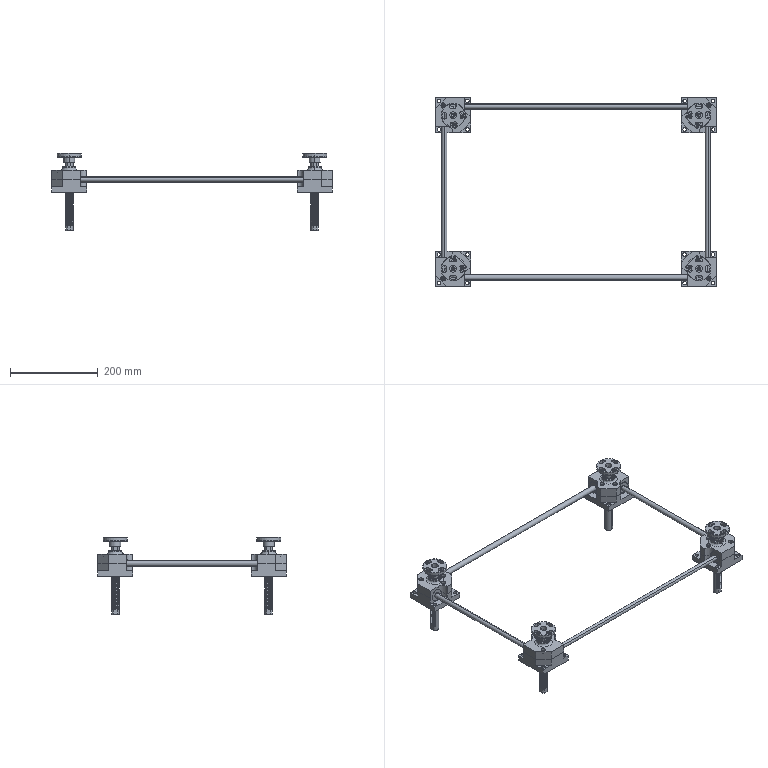Part | SolidWorks | 180 solids | 7268 faces | volume 1356586 mm3 | cylinder 3488 | plane 2080 | sphere 864 | cone 580 | torus 256 | commonest cylinder face diameters 0.5 x912 0.76 x608 13.128 x400 19.2 x200 20.8 x200 26 x200